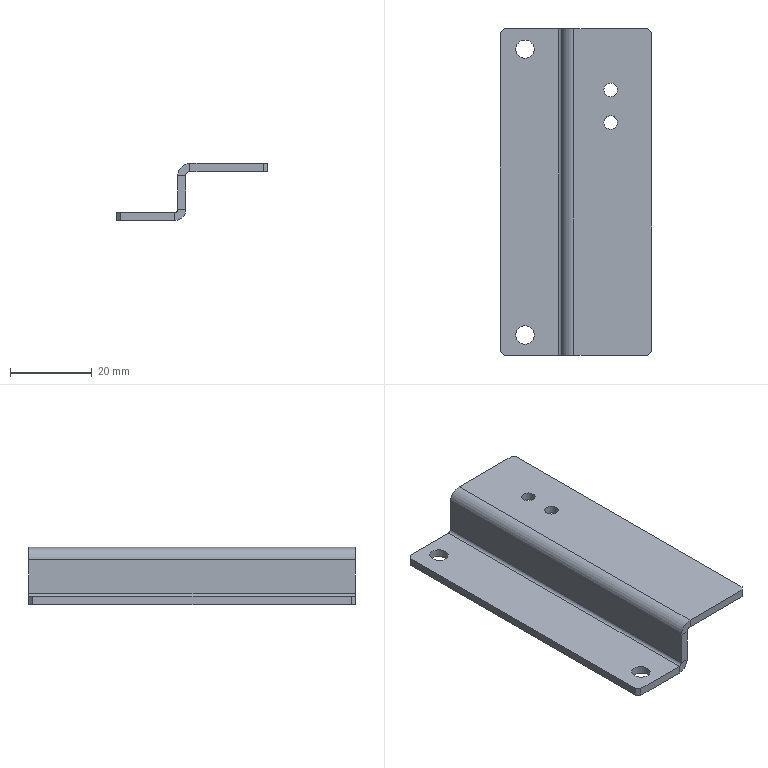Part | NX | 1 solid | 30 faces | box 37 x 80 x 14 mm | volume 7482 mm3 | plane 22 | cylinder 8 | commonest cylinder face diameters 3.3 x2 4.5 x2 1.473 x1 2 x1 5.473 x1 6 x1
STEP:
#1=CARTESIAN_POINT('',(-12.,-40.,-3.));
#2=VERTEX_POINT('',#1);
#3=CARTESIAN_POINT('',(-12.,-40.,-11.263));
#4=VERTEX_POINT('',#3);
#5=CARTESIAN_POINT('',(-12.,-40.,-12.));
#6=DIRECTION('',(0.,0.,-1.));
#7=VECTOR('',#6,1000.);
#8=LINE('',#5,#7);
#9=EDGE_CURVE('',#2,#4,#8,.T.);
#10=ORIENTED_EDGE('',*,*,#9,.T.);
#11=CARTESIAN_POINT('',(-10.,-40.,-11.263));
#12=VERTEX_POINT('',#11);
#13=CARTESIAN_POINT('',(-12.,-40.,-11.263));
#14=DIRECTION('',(1.,0.,0.));
#15=VECTOR('',#14,1000.);
#16=LINE('',#13,#15);
#17=EDGE_CURVE('',#4,#12,#16,.T.);
#18=ORIENTED_EDGE('',*,*,#17,.T.);
#19=CARTESIAN_POINT('',(-10.,-40.,-3.));
#20=VERTEX_POINT('',#19);
#21=CARTESIAN_POINT('',(-10.,-40.,-12.));
#22=DIRECTION('',(0.,0.,-1.));
#23=VECTOR('',#22,1000.);
#24=LINE('',#21,#23);
#25=EDGE_CURVE('',#20,#12,#24,.T.);
#26=ORIENTED_EDGE('',*,*,#25,.F.);
#27=CARTESIAN_POINT('',(-10.,-40.,-3.));
#28=DIRECTION('',(-1.,0.,0.));
#29=VECTOR('',#28,1000.);
#30=LINE('',#27,#29);
#31=EDGE_CURVE('',#20,#2,#30,.T.);
#32=ORIENTED_EDGE('',*,*,#31,.T.);
#33=EDGE_LOOP('',(#10,#18,#26,#32));
#34=FACE_BOUND('',#33,.T.);
#35=CARTESIAN_POINT('',(-12.,-40.,-12.));
#36=DIRECTION('',(0.,-1.,0.));
#37=DIRECTION('',(0.,0.,-1.));
#38=AXIS2_PLACEMENT_3D('',#35,#36,#37);
#39=PLANE('',#38);
#40=ADVANCED_FACE('',(#34),#39,.T.);
#41=CARTESIAN_POINT('',(-12.,40.,-11.263));
#42=VERTEX_POINT('',#41);
#43=CARTESIAN_POINT('',(-12.,40.,-3.));
#44=VERTEX_POINT('',#43);
#45=CARTESIAN_POINT('',(-12.,40.,-2.));
#46=DIRECTION('',(0.,0.,1.));
#47=VECTOR('',#46,1000.);
#48=LINE('',#45,#47);
#49=EDGE_CURVE('',#42,#44,#48,.T.);
#50=ORIENTED_EDGE('',*,*,#49,.F.);
#51=CARTESIAN_POINT('',(-12.,-40.,-11.263));
#52=DIRECTION('',(0.,-1.,0.));
#53=VECTOR('',#52,1000.);
#54=LINE('',#51,#53);
#55=EDGE_CURVE('',#4,#42,#54,.F.);
#56=ORIENTED_EDGE('',*,*,#55,.F.);
#57=ORIENTED_EDGE('',*,*,#9,.F.);
#58=CARTESIAN_POINT('',(-12.,0.,-3.));
#59=DIRECTION('',(0.,1.,0.));
#60=VECTOR('',#59,1000.);
#61=LINE('',#58,#60);
#62=EDGE_CURVE('',#2,#44,#61,.T.);
#63=ORIENTED_EDGE('',*,*,#62,.T.);
#64=EDGE_LOOP('',(#50,#56,#57,#63));
#65=FACE_BOUND('',#64,.T.);
#66=CARTESIAN_POINT('',(-12.,0.,0.));
#67=DIRECTION('',(-1.,0.,0.));
#68=DIRECTION('',(0.,0.,1.));
#69=AXIS2_PLACEMENT_3D('',#66,#67,#68);
#70=PLANE('',#69);
#71=ADVANCED_FACE('',(#65),#70,.T.);
#72=CARTESIAN_POINT('',(-10.,40.,-11.263));
#73=VERTEX_POINT('',#72);
#74=CARTESIAN_POINT('',(-10.,-40.,-11.263));
#75=DIRECTION('',(0.,-1.,0.));
#76=VECTOR('',#75,1000.);
#77=LINE('',#74,#76);
#78=EDGE_CURVE('',#12,#73,#77,.F.);
#79=ORIENTED_EDGE('',*,*,#78,.T.);
#80=CARTESIAN_POINT('',(-10.,40.,-3.));
#81=VERTEX_POINT('',#80);
#82=CARTESIAN_POINT('',(-10.,40.,-2.));
#83=DIRECTION('',(0.,0.,1.));
#84=VECTOR('',#83,1000.);
#85=LINE('',#82,#84);
#86=EDGE_CURVE('',#73,#81,#85,.T.);
#87=ORIENTED_EDGE('',*,*,#86,.T.);
#88=CARTESIAN_POINT('',(-10.,-40.,-3.));
#89=DIRECTION('',(0.,1.,0.));
#90=VECTOR('',#89,1000.);
#91=LINE('',#88,#90);
#92=EDGE_CURVE('',#20,#81,#91,.T.);
#93=ORIENTED_EDGE('',*,*,#92,.F.);
#94=ORIENTED_EDGE('',*,*,#25,.T.);
#95=EDGE_LOOP('',(#79,#87,#93,#94));
#96=FACE_BOUND('',#95,.T.);
#97=CARTESIAN_POINT('',(-10.,0.,0.));
#98=DIRECTION('',(-1.,0.,0.));
#99=DIRECTION('',(0.,0.,1.));
#100=AXIS2_PLACEMENT_3D('',#97,#98,#99);
#101=PLANE('',#100);
#102=ADVANCED_FACE('',(#96),#101,.F.);
#103=CARTESIAN_POINT('',(9.,40.,0.));
#104=VERTEX_POINT('',#103);
#105=CARTESIAN_POINT('',(-9.,40.,0.));
#106=VERTEX_POINT('',#105);
#107=CARTESIAN_POINT('',(-10.,40.,0.));
#108=DIRECTION('',(-1.,0.,0.));
#109=VECTOR('',#108,1000.);
#110=LINE('',#107,#109);
#111=EDGE_CURVE('',#104,#106,#110,.T.);
#112=ORIENTED_EDGE('',*,*,#111,.F.);
#113=CARTESIAN_POINT('',(9.,40.,-2.));
#114=VERTEX_POINT('',#113);
#115=CARTESIAN_POINT('',(9.,40.,-2.));
#116=DIRECTION('',(0.,0.,-1.));
#117=VECTOR('',#116,1000.);
#118=LINE('',#115,#117);
#119=EDGE_CURVE('',#104,#114,#118,.T.);
#120=ORIENTED_EDGE('',*,*,#119,.T.);
#121=CARTESIAN_POINT('',(-9.,40.,-2.));
#122=VERTEX_POINT('',#121);
#123=CARTESIAN_POINT('',(-10.,40.,-2.));
#124=DIRECTION('',(-1.,0.,0.));
#125=VECTOR('',#124,1000.);
#126=LINE('',#123,#125);
#127=EDGE_CURVE('',#114,#122,#126,.T.);
#128=ORIENTED_EDGE('',*,*,#127,.T.);
#129=CARTESIAN_POINT('',(-9.,40.,-2.));
#130=DIRECTION('',(0.,0.,1.));
#131=VECTOR('',#130,1000.);
#132=LINE('',#129,#131);
#133=EDGE_CURVE('',#122,#106,#132,.T.);
#134=ORIENTED_EDGE('',*,*,#133,.T.);
#135=EDGE_LOOP('',(#112,#120,#128,#134));
#136=FACE_BOUND('',#135,.T.);
#137=CARTESIAN_POINT('',(-10.,40.,-2.));
#138=DIRECTION('',(0.,1.,0.));
#139=DIRECTION('',(0.,0.,1.));
#140=AXIS2_PLACEMENT_3D('',#137,#138,#139);
#141=PLANE('',#140);
#142=ADVANCED_FACE('',(#136),#141,.T.);
#143=CARTESIAN_POINT('',(1.65,17.,-2.));
#144=VERTEX_POINT('',#143);
#145=CARTESIAN_POINT('',(0.,17.,-2.));
#146=DIRECTION('',(0.,0.,1.));
#147=DIRECTION('',(1.,0.,0.));
#148=AXIS2_PLACEMENT_3D('',#145,#146,#147);
#149=CIRCLE('',#148,1.65);
#150=EDGE_CURVE('',#144,#144,#149,.T.);
#151=ORIENTED_EDGE('',*,*,#150,.T.);
#152=EDGE_LOOP('',(#151));
#153=FACE_BOUND('',#152,.T.);
#154=CARTESIAN_POINT('',(1.65,25.,-2.));
#155=VERTEX_POINT('',#154);
#156=CARTESIAN_POINT('',(0.,25.,-2.));
#157=DIRECTION('',(0.,0.,1.));
#158=DIRECTION('',(1.,0.,0.));
#159=AXIS2_PLACEMENT_3D('',#156,#157,#158);
#160=CIRCLE('',#159,1.65);
#161=EDGE_CURVE('',#155,#155,#160,.T.);
#162=ORIENTED_EDGE('',*,*,#161,.T.);
#163=EDGE_LOOP('',(#162));
#164=FACE_BOUND('',#163,.T.);
#165=CARTESIAN_POINT('',(10.,-39.,-2.));
#166=VERTEX_POINT('',#165);
#167=CARTESIAN_POINT('',(10.,39.,-2.));
#168=VERTEX_POINT('',#167);
#169=CARTESIAN_POINT('',(10.,-40.,-2.));
#170=DIRECTION('',(0.,1.,0.));
#171=VECTOR('',#170,1000.);
#172=LINE('',#169,#171);
#173=EDGE_CURVE('',#166,#168,#172,.T.);
#174=ORIENTED_EDGE('',*,*,#173,.F.);
#175=CARTESIAN_POINT('',(9.,-40.,-2.));
#176=VERTEX_POINT('',#175);
#177=CARTESIAN_POINT('',(24.5,-24.5,-2.));
#178=DIRECTION('',(0.7071,0.7071,0.));
#179=VECTOR('',#178,1000.);
#180=LINE('',#177,#179);
#181=EDGE_CURVE('',#166,#176,#180,.F.);
#182=ORIENTED_EDGE('',*,*,#181,.T.);
#183=CARTESIAN_POINT('',(-9.,-40.,-2.));
#184=VERTEX_POINT('',#183);
#185=CARTESIAN_POINT('',(-10.,-40.,-2.));
#186=DIRECTION('',(1.,0.,0.));
#187=VECTOR('',#186,1000.);
#188=LINE('',#185,#187);
#189=EDGE_CURVE('',#184,#176,#188,.T.);
#190=ORIENTED_EDGE('',*,*,#189,.F.);
#191=CARTESIAN_POINT('',(-9.,40.,-2.));
#192=DIRECTION('',(0.,1.,0.));
#193=VECTOR('',#192,1000.);
#194=LINE('',#191,#193);
#195=EDGE_CURVE('',#122,#184,#194,.F.);
#196=ORIENTED_EDGE('',*,*,#195,.F.);
#197=ORIENTED_EDGE('',*,*,#127,.F.);
#198=CARTESIAN_POINT('',(24.5,24.5,-2.));
#199=DIRECTION('',(-0.7071,0.7071,0.));
#200=VECTOR('',#199,1000.);
#201=LINE('',#198,#200);
#202=EDGE_CURVE('',#114,#168,#201,.F.);
#203=ORIENTED_EDGE('',*,*,#202,.T.);
#204=EDGE_LOOP('',(#174,#182,#190,#196,#197,#203));
#205=FACE_BOUND('',#204,.T.);
#206=CARTESIAN_POINT('',(0.,0.,-2.));
#207=DIRECTION('',(0.,0.,-1.));
#208=DIRECTION('',(-1.,0.,0.));
#209=AXIS2_PLACEMENT_3D('',#206,#207,#208);
#210=PLANE('',#209);
#211=ADVANCED_FACE('',(#153,#164,#205),#210,.T.);
#212=CARTESIAN_POINT('',(1.65,17.,0.));
#213=VERTEX_POINT('',#212);
#214=CARTESIAN_POINT('',(0.,17.,0.));
#215=DIRECTION('',(0.,0.,1.));
#216=DIRECTION('',(1.,0.,0.));
#217=AXIS2_PLACEMENT_3D('',#214,#215,#216);
#218=CIRCLE('',#217,1.65);
#219=EDGE_CURVE('',#213,#213,#218,.T.);
#220=ORIENTED_EDGE('',*,*,#219,.F.);
#221=EDGE_LOOP('',(#220));
#222=FACE_BOUND('',#221,.T.);
#223=CARTESIAN_POINT('',(1.65,25.,0.));
#224=VERTEX_POINT('',#223);
#225=CARTESIAN_POINT('',(0.,25.,0.));
#226=DIRECTION('',(0.,0.,1.));
#227=DIRECTION('',(1.,0.,0.));
#228=AXIS2_PLACEMENT_3D('',#225,#226,#227);
#229=CIRCLE('',#228,1.65);
#230=EDGE_CURVE('',#224,#224,#229,.T.);
#231=ORIENTED_EDGE('',*,*,#230,.F.);
#232=EDGE_LOOP('',(#231));
#233=FACE_BOUND('',#232,.T.);
#234=CARTESIAN_POINT('',(-9.,-40.,0.));
#235=VERTEX_POINT('',#234);
#236=CARTESIAN_POINT('',(9.,-40.,0.));
#237=VERTEX_POINT('',#236);
#238=CARTESIAN_POINT('',(-10.,-40.,0.));
#239=DIRECTION('',(1.,0.,0.));
#240=VECTOR('',#239,1000.);
#241=LINE('',#238,#240);
#242=EDGE_CURVE('',#235,#237,#241,.T.);
#243=ORIENTED_EDGE('',*,*,#242,.T.);
#244=CARTESIAN_POINT('',(10.,-39.,0.));
#245=VERTEX_POINT('',#244);
#246=CARTESIAN_POINT('',(9.,-40.,0.));
#247=DIRECTION('',(-0.7071,-0.7071,0.));
#248=VECTOR('',#247,1000.);
#249=LINE('',#246,#248);
#250=EDGE_CURVE('',#237,#245,#249,.F.);
#251=ORIENTED_EDGE('',*,*,#250,.T.);
#252=CARTESIAN_POINT('',(10.,39.,0.));
#253=VERTEX_POINT('',#252);
#254=CARTESIAN_POINT('',(10.,-40.,0.));
#255=DIRECTION('',(0.,1.,0.));
#256=VECTOR('',#255,1000.);
#257=LINE('',#254,#256);
#258=EDGE_CURVE('',#245,#253,#257,.T.);
#259=ORIENTED_EDGE('',*,*,#258,.T.);
#260=CARTESIAN_POINT('',(10.,39.,0.));
#261=DIRECTION('',(0.7071,-0.7071,0.));
#262=VECTOR('',#261,1000.);
#263=LINE('',#260,#262);
#264=EDGE_CURVE('',#253,#104,#263,.F.);
#265=ORIENTED_EDGE('',*,*,#264,.T.);
#266=ORIENTED_EDGE('',*,*,#111,.T.);
#267=CARTESIAN_POINT('',(-9.,40.,0.));
#268=DIRECTION('',(0.,1.,0.));
#269=VECTOR('',#268,1000.);
#270=LINE('',#267,#269);
#271=EDGE_CURVE('',#106,#235,#270,.F.);
#272=ORIENTED_EDGE('',*,*,#271,.T.);
#273=EDGE_LOOP('',(#243,#251,#259,#265,#266,#272));
#274=FACE_BOUND('',#273,.T.);
#275=CARTESIAN_POINT('',(0.,0.,0.));
#276=DIRECTION('',(0.,0.,-1.));
#277=DIRECTION('',(-1.,0.,0.));
#278=AXIS2_PLACEMENT_3D('',#275,#276,#277);
#279=PLANE('',#278);
#280=ADVANCED_FACE('',(#222,#233,#274),#279,.F.);
#281=ORIENTED_EDGE('',*,*,#258,.F.);
#282=CARTESIAN_POINT('',(10.,-39.,-2.));
#283=DIRECTION('',(0.,0.,-1.));
#284=VECTOR('',#283,1000.);
#285=LINE('',#282,#284);
#286=EDGE_CURVE('',#245,#166,#285,.T.);
#287=ORIENTED_EDGE('',*,*,#286,.T.);
#288=ORIENTED_EDGE('',*,*,#173,.T.);
#289=CARTESIAN_POINT('',(10.,39.,-2.));
#290=DIRECTION('',(0.,0.,1.));
#291=VECTOR('',#290,1000.);
#292=LINE('',#289,#291);
#293=EDGE_CURVE('',#168,#253,#292,.T.);
#294=ORIENTED_EDGE('',*,*,#293,.T.);
#295=EDGE_LOOP('',(#281,#287,#288,#294));
#296=FACE_BOUND('',#295,.T.);
#297=CARTESIAN_POINT('',(10.,-40.,-2.));
#298=DIRECTION('',(1.,0.,0.));
#299=DIRECTION('',(0.,0.,-1.));
#300=AXIS2_PLACEMENT_3D('',#297,#298,#299);
#301=PLANE('',#300);
#302=ADVANCED_FACE('',(#296),#301,.T.);
#303=ORIENTED_EDGE('',*,*,#189,.T.);
#304=CARTESIAN_POINT('',(9.,-40.,-2.));
#305=DIRECTION('',(0.,0.,1.));
#306=VECTOR('',#305,1000.);
#307=LINE('',#304,#306);
#308=EDGE_CURVE('',#176,#237,#307,.T.);
#309=ORIENTED_EDGE('',*,*,#308,.T.);
#310=ORIENTED_EDGE('',*,*,#242,.F.);
#311=CARTESIAN_POINT('',(-9.,-40.,-2.));
#312=DIRECTION('',(0.,0.,1.));
#313=VECTOR('',#312,1000.);
#314=LINE('',#311,#313);
#315=EDGE_CURVE('',#184,#235,#314,.T.);
#316=ORIENTED_EDGE('',*,*,#315,.F.);
#317=EDGE_LOOP('',(#303,#309,#310,#316));
#318=FACE_BOUND('',#317,.T.);
#319=CARTESIAN_POINT('',(-10.,-40.,-2.));
#320=DIRECTION('',(0.,-1.,0.));
#321=DIRECTION('',(0.,0.,-1.));
#322=AXIS2_PLACEMENT_3D('',#319,#320,#321);
#323=PLANE('',#322);
#324=ADVANCED_FACE('',(#318),#323,.T.);
#325=ORIENTED_EDGE('',*,*,#150,.F.);
#326=EDGE_LOOP('',(#325));
#327=FACE_BOUND('',#326,.T.);
#328=ORIENTED_EDGE('',*,*,#219,.T.);
#329=EDGE_LOOP('',(#328));
#330=FACE_BOUND('',#329,.T.);
#331=CARTESIAN_POINT('',(0.,17.,0.));
#332=DIRECTION('',(0.,0.,1.));
#333=DIRECTION('',(1.,0.,0.));
#334=AXIS2_PLACEMENT_3D('',#331,#332,#333);
#335=CYLINDRICAL_SURFACE('',#334,1.65);
#336=ADVANCED_FACE('',(#327,#330),#335,.F.);
#337=ORIENTED_EDGE('',*,*,#161,.F.);
#338=EDGE_LOOP('',(#337));
#339=FACE_BOUND('',#338,.T.);
#340=ORIENTED_EDGE('',*,*,#230,.T.);
#341=EDGE_LOOP('',(#340));
#342=FACE_BOUND('',#341,.T.);
#343=CARTESIAN_POINT('',(0.,25.,0.));
#344=DIRECTION('',(0.,0.,1.));
#345=DIRECTION('',(1.,0.,0.));
#346=AXIS2_PLACEMENT_3D('',#343,#344,#345);
#347=CYLINDRICAL_SURFACE('',#346,1.65);
#348=ADVANCED_FACE('',(#339,#342),#347,.F.);
#349=ORIENTED_EDGE('',*,*,#31,.F.);
#350=CARTESIAN_POINT('',(-9.,-40.,-3.));
#351=DIRECTION('',(0.,1.,0.));
#352=DIRECTION('',(0.,0.,1.));
#353=AXIS2_PLACEMENT_3D('',#350,#351,#352);
#354=CIRCLE('',#353,1.);
#355=EDGE_CURVE('',#184,#20,#354,.F.);
#356=ORIENTED_EDGE('',*,*,#355,.F.);
#357=ORIENTED_EDGE('',*,*,#315,.T.);
#358=CARTESIAN_POINT('',(-9.,-40.,-3.));
#359=DIRECTION('',(0.,1.,0.));
#360=DIRECTION('',(0.,0.,1.));
#361=AXIS2_PLACEMENT_3D('',#358,#359,#360);
#362=CIRCLE('',#361,3.);
#363=EDGE_CURVE('',#235,#2,#362,.F.);
#364=ORIENTED_EDGE('',*,*,#363,.T.);
#365=EDGE_LOOP('',(#349,#356,#357,#364));
#366=FACE_BOUND('',#365,.T.);
#367=CARTESIAN_POINT('',(-9.,-40.,-3.));
#368=DIRECTION('',(0.,-1.,0.));
#369=DIRECTION('',(0.,0.,-1.));
#370=AXIS2_PLACEMENT_3D('',#367,#368,#369);
#371=PLANE('',#370);
#372=ADVANCED_FACE('',(#366),#371,.T.);
#373=CARTESIAN_POINT('',(-9.,40.,-3.));
#374=DIRECTION('',(0.,1.,0.));
#375=DIRECTION('',(0.,0.,1.));
#376=AXIS2_PLACEMENT_3D('',#373,#374,#375);
#377=CIRCLE('',#376,1.);
#378=EDGE_CURVE('',#81,#122,#377,.T.);
#379=ORIENTED_EDGE('',*,*,#378,.F.);
#380=CARTESIAN_POINT('',(-10.,40.,-3.));
#381=DIRECTION('',(-1.,0.,0.));
#382=VECTOR('',#381,1000.);
#383=LINE('',#380,#382);
#384=EDGE_CURVE('',#81,#44,#383,.T.);
#385=ORIENTED_EDGE('',*,*,#384,.T.);
#386=CARTESIAN_POINT('',(-9.,40.,-3.));
#387=DIRECTION('',(0.,1.,0.));
#388=DIRECTION('',(0.,0.,1.));
#389=AXIS2_PLACEMENT_3D('',#386,#387,#388);
#390=CIRCLE('',#389,3.);
#391=EDGE_CURVE('',#44,#106,#390,.T.);
#392=ORIENTED_EDGE('',*,*,#391,.T.);
#393=ORIENTED_EDGE('',*,*,#133,.F.);
#394=EDGE_LOOP('',(#379,#385,#392,#393));
#395=FACE_BOUND('',#394,.T.);
#396=CARTESIAN_POINT('',(-9.,40.,-3.));
#397=DIRECTION('',(0.,-1.,0.));
#398=DIRECTION('',(0.,0.,-1.));
#399=AXIS2_PLACEMENT_3D('',#396,#397,#398);
#400=PLANE('',#399);
#401=ADVANCED_FACE('',(#395),#400,.F.);
#402=ORIENTED_EDGE('',*,*,#271,.F.);
#403=ORIENTED_EDGE('',*,*,#391,.F.);
#404=ORIENTED_EDGE('',*,*,#62,.F.);
#405=ORIENTED_EDGE('',*,*,#363,.F.);
#406=EDGE_LOOP('',(#402,#403,#404,#405));
#407=FACE_BOUND('',#406,.T.);
#408=CARTESIAN_POINT('',(-9.,40.,-3.));
#409=DIRECTION('',(0.,1.,0.));
#410=DIRECTION('',(-1.,0.,0.));
#411=AXIS2_PLACEMENT_3D('',#408,#409,#410);
#412=CYLINDRICAL_SURFACE('',#411,3.);
#413=ADVANCED_FACE('',(#407),#412,.T.);
#414=ORIENTED_EDGE('',*,*,#195,.T.);
#415=ORIENTED_EDGE('',*,*,#355,.T.);
#416=ORIENTED_EDGE('',*,*,#92,.T.);
#417=ORIENTED_EDGE('',*,*,#378,.T.);
#418=EDGE_LOOP('',(#414,#415,#416,#417));
#419=FACE_BOUND('',#418,.T.);
#420=CARTESIAN_POINT('',(-9.,40.,-3.));
#421=DIRECTION('',(0.,1.,0.));
#422=DIRECTION('',(-1.,0.,0.));
#423=AXIS2_PLACEMENT_3D('',#420,#421,#422);
#424=CYLINDRICAL_SURFACE('',#423,1.);
#425=ADVANCED_FACE('',(#419),#424,.F.);
#426=CARTESIAN_POINT('',(-12.,40.,-11.263));
#427=DIRECTION('',(1.,0.,0.));
#428=VECTOR('',#427,1000.);
#429=LINE('',#426,#428);
#430=EDGE_CURVE('',#42,#73,#429,.T.);
#431=ORIENTED_EDGE('',*,*,#430,.F.);
#432=ORIENTED_EDGE('',*,*,#49,.T.);
#433=ORIENTED_EDGE('',*,*,#384,.F.);
#434=ORIENTED_EDGE('',*,*,#86,.F.);
#435=EDGE_LOOP('',(#431,#432,#433,#434));
#436=FACE_BOUND('',#435,.T.);
#437=CARTESIAN_POINT('',(-12.,40.,-2.));
#438=DIRECTION('',(0.,1.,0.));
#439=DIRECTION('',(0.,0.,1.));
#440=AXIS2_PLACEMENT_3D('',#437,#438,#439);
#441=PLANE('',#440);
#442=ADVANCED_FACE('',(#436),#441,.T.);
#443=CARTESIAN_POINT('',(-12.737,40.,-12.));
#444=VERTEX_POINT('',#443);
#445=CARTESIAN_POINT('',(-12.737,40.,-14.));
#446=VERTEX_POINT('',#445);
#447=CARTESIAN_POINT('',(-12.737,40.,-12.));
#448=DIRECTION('',(0.,0.,-1.));
#449=VECTOR('',#448,1000.);
#450=LINE('',#447,#449);
#451=EDGE_CURVE('',#444,#446,#450,.T.);
#452=ORIENTED_EDGE('',*,*,#451,.F.);
#453=CARTESIAN_POINT('',(-12.737,40.,-11.263));
#454=DIRECTION('',(0.,-1.,0.));
#455=DIRECTION('',(0.,0.,-1.));
#456=AXIS2_PLACEMENT_3D('',#453,#454,#455);
#457=CIRCLE('',#456,0.7366);
#458=EDGE_CURVE('',#42,#444,#457,.F.);
#459=ORIENTED_EDGE('',*,*,#458,.F.);
#460=ORIENTED_EDGE('',*,*,#430,.T.);
#461=CARTESIAN_POINT('',(-12.737,40.,-11.263));
#462=DIRECTION('',(0.,-1.,0.));
#463=DIRECTION('',(0.,0.,-1.));
#464=AXIS2_PLACEMENT_3D('',#461,#462,#463);
#465=CIRCLE('',#464,2.737);
#466=EDGE_CURVE('',#73,#446,#465,.F.);
#467=ORIENTED_EDGE('',*,*,#466,.T.);
#468=EDGE_LOOP('',(#452,#459,#460,#467));
#469=FACE_BOUND('',#468,.T.);
#470=CARTESIAN_POINT('',(-12.737,40.,-11.263));
#471=DIRECTION('',(0.,1.,0.));
#472=DIRECTION('',(0.,0.,1.));
#473=AXIS2_PLACEMENT_3D('',#470,#471,#472);
#474=PLANE('',#473);
#475=ADVANCED_FACE('',(#469),#474,.T.);
#476=CARTESIAN_POINT('',(-12.737,-40.,-12.));
#477=VERTEX_POINT('',#476);
#478=CARTESIAN_POINT('',(-12.737,-40.,-11.263));
#479=DIRECTION('',(0.,-1.,0.));
#480=DIRECTION('',(0.,0.,-1.));
#481=AXIS2_PLACEMENT_3D('',#478,#479,#480);
#482=CIRCLE('',#481,0.7366);
#483=EDGE_CURVE('',#477,#4,#482,.T.);
#484=ORIENTED_EDGE('',*,*,#483,.F.);
#485=CARTESIAN_POINT('',(-12.737,-40.,-14.));
#486=VERTEX_POINT('',#485);
#487=CARTESIAN_POINT('',(-12.737,-40.,-12.));
#488=DIRECTION('',(0.,0.,-1.));
#489=VECTOR('',#488,1000.);
#490=LINE('',#487,#489);
#491=EDGE_CURVE('',#477,#486,#490,.T.);
#492=ORIENTED_EDGE('',*,*,#491,.T.);
#493=CARTESIAN_POINT('',(-12.737,-40.,-11.263));
#494=DIRECTION('',(0.,-1.,0.));
#495=DIRECTION('',(0.,0.,-1.));
#496=AXIS2_PLACEMENT_3D('',#493,#494,#495);
#497=CIRCLE('',#496,2.737);
#498=EDGE_CURVE('',#486,#12,#497,.T.);
#499=ORIENTED_EDGE('',*,*,#498,.T.);
#500=ORIENTED_EDGE('',*,*,#17,.F.);
#501=EDGE_LOOP('',(#484,#492,#499,#500));
#502=FACE_BOUND('',#501,.T.);
#503=CARTESIAN_POINT('',(-12.737,-40.,-11.263));
#504=DIRECTION('',(0.,1.,0.));
#505=DIRECTION('',(0.,0.,1.));
#506=AXIS2_PLACEMENT_3D('',#503,#504,#505);
#507=PLANE('',#506);
#508=ADVANCED_FACE('',(#502),#507,.F.);
#509=ORIENTED_EDGE('',*,*,#78,.F.);
#510=ORIENTED_EDGE('',*,*,#498,.F.);
#511=CARTESIAN_POINT('',(-12.737,0.,-14.));
#512=DIRECTION('',(0.,-1.,0.));
#513=VECTOR('',#512,1000.);
#514=LINE('',#511,#513);
#515=EDGE_CURVE('',#446,#486,#514,.T.);
#516=ORIENTED_EDGE('',*,*,#515,.F.);
#517=ORIENTED_EDGE('',*,*,#466,.F.);
#518=EDGE_LOOP('',(#509,#510,#516,#517));
#519=FACE_BOUND('',#518,.T.);
#520=CARTESIAN_POINT('',(-12.737,-40.,-11.263));
#521=DIRECTION('',(0.,-1.,0.));
#522=DIRECTION('',(0.,0.,-1.));
#523=AXIS2_PLACEMENT_3D('',#520,#521,#522);
#524=CYLINDRICAL_SURFACE('',#523,2.737);
#525=ADVANCED_FACE('',(#519),#524,.T.);
#526=ORIENTED_EDGE('',*,*,#55,.T.);
#527=ORIENTED_EDGE('',*,*,#458,.T.);
#528=CARTESIAN_POINT('',(-12.737,40.,-12.));
#529=DIRECTION('',(0.,-1.,0.));
#530=VECTOR('',#529,1000.);
#531=LINE('',#528,#530);
#532=EDGE_CURVE('',#444,#477,#531,.T.);
#533=ORIENTED_EDGE('',*,*,#532,.T.);
#534=ORIENTED_EDGE('',*,*,#483,.T.);
#535=EDGE_LOOP('',(#526,#527,#533,#534));
#536=FACE_BOUND('',#535,.T.);
#537=CARTESIAN_POINT('',(-12.737,-40.,-11.263));
#538=DIRECTION('',(0.,-1.,0.));
#539=DIRECTION('',(0.,0.,-1.));
#540=AXIS2_PLACEMENT_3D('',#537,#538,#539);
#541=CYLINDRICAL_SURFACE('',#540,0.7366);
#542=ADVANCED_FACE('',(#536),#541,.F.);
#543=CARTESIAN_POINT('',(-26.,-40.,-12.));
#544=VERTEX_POINT('',#543);
#545=CARTESIAN_POINT('',(-12.,-40.,-12.));
#546=DIRECTION('',(1.,0.,0.));
#547=VECTOR('',#546,1000.);
#548=LINE('',#545,#547);
#549=EDGE_CURVE('',#544,#477,#548,.T.);
#550=ORIENTED_EDGE('',*,*,#549,.F.);
#551=CARTESIAN_POINT('',(-26.,-40.,-14.));
#552=VERTEX_POINT('',#551);
#553=CARTESIAN_POINT('',(-26.,-40.,-14.));
#554=DIRECTION('',(0.,0.,-1.));
#555=VECTOR('',#554,1000.);
#556=LINE('',#553,#555);
#557=EDGE_CURVE('',#544,#552,#556,.T.);
#558=ORIENTED_EDGE('',*,*,#557,.T.);
#559=CARTESIAN_POINT('',(-12.,-40.,-14.));
#560=DIRECTION('',(1.,0.,0.));
#561=VECTOR('',#560,1000.);
#562=LINE('',#559,#561);
#563=EDGE_CURVE('',#552,#486,#562,.T.);
#564=ORIENTED_EDGE('',*,*,#563,.T.);
#565=ORIENTED_EDGE('',*,*,#491,.F.);
#566=EDGE_LOOP('',(#550,#558,#564,#565));
#567=FACE_BOUND('',#566,.T.);
#568=CARTESIAN_POINT('',(-12.,-40.,-14.));
#569=DIRECTION('',(0.,-1.,0.));
#570=DIRECTION('',(0.,0.,-1.));
#571=AXIS2_PLACEMENT_3D('',#568,#569,#570);
#572=PLANE('',#571);
#573=ADVANCED_FACE('',(#567),#572,.T.);
#574=CARTESIAN_POINT('',(-26.,40.,-14.));
#575=VERTEX_POINT('',#574);
#576=CARTESIAN_POINT('',(-27.,40.,-14.));
#577=DIRECTION('',(-1.,0.,0.));
#578=VECTOR('',#577,1000.);
#579=LINE('',#576,#578);
#580=EDGE_CURVE('',#446,#575,#579,.T.);
#581=ORIENTED_EDGE('',*,*,#580,.T.);
#582=CARTESIAN_POINT('',(-26.,40.,-12.));
#583=VERTEX_POINT('',#582);
#584=CARTESIAN_POINT('',(-26.,40.,-14.));
#585=DIRECTION('',(0.,0.,1.));
#586=VECTOR('',#585,1000.);
#587=LINE('',#584,#586);
#588=EDGE_CURVE('',#575,#583,#587,.T.);
#589=ORIENTED_EDGE('',*,*,#588,.T.);
#590=CARTESIAN_POINT('',(-27.,40.,-12.));
#591=DIRECTION('',(-1.,0.,0.));
#592=VECTOR('',#591,1000.);
#593=LINE('',#590,#592);
#594=EDGE_CURVE('',#444,#583,#593,.T.);
#595=ORIENTED_EDGE('',*,*,#594,.F.);
#596=ORIENTED_EDGE('',*,*,#451,.T.);
#597=EDGE_LOOP('',(#581,#589,#595,#596));
#598=FACE_BOUND('',#597,.T.);
#599=CARTESIAN_POINT('',(-27.,40.,-14.));
#600=DIRECTION('',(0.,1.,0.));
#601=DIRECTION('',(-1.,0.,0.));
#602=AXIS2_PLACEMENT_3D('',#599,#600,#601);
#603=PLANE('',#602);
#604=ADVANCED_FACE('',(#598),#603,.T.);
#605=CARTESIAN_POINT('',(-23.25,35.,-14.));
#606=VERTEX_POINT('',#605);
#607=CARTESIAN_POINT('',(-21.,35.,-14.));
#608=DIRECTION('',(0.,0.,-1.));
#609=DIRECTION('',(-1.,0.,0.));
#610=AXIS2_PLACEMENT_3D('',#607,#608,#609);
#611=CIRCLE('',#610,2.25);
#612=EDGE_CURVE('',#606,#606,#611,.T.);
#613=ORIENTED_EDGE('',*,*,#612,.F.);
#614=EDGE_LOOP('',(#613));
#615=FACE_BOUND('',#614,.T.);
#616=CARTESIAN_POINT('',(-23.25,-35.,-14.));
#617=VERTEX_POINT('',#616);
#618=CARTESIAN_POINT('',(-21.,-35.,-14.));
#619=DIRECTION('',(0.,0.,-1.));
#620=DIRECTION('',(-1.,0.,0.));
#621=AXIS2_PLACEMENT_3D('',#618,#619,#620);
#622=CIRCLE('',#621,2.25);
#623=EDGE_CURVE('',#617,#617,#622,.T.);
#624=ORIENTED_EDGE('',*,*,#623,.F.);
#625=EDGE_LOOP('',(#624));
#626=FACE_BOUND('',#625,.T.);
#627=CARTESIAN_POINT('',(-27.,39.,-14.));
#628=VERTEX_POINT('',#627);
#629=CARTESIAN_POINT('',(-27.,-39.,-14.));
#630=VERTEX_POINT('',#629);
#631=CARTESIAN_POINT('',(-27.,-40.,-14.));
#632=DIRECTION('',(0.,-1.,0.));
#633=VECTOR('',#632,1000.);
#634=LINE('',#631,#633);
#635=EDGE_CURVE('',#628,#630,#634,.T.);
#636=ORIENTED_EDGE('',*,*,#635,.F.);
#637=CARTESIAN_POINT('',(-33.,33.,-14.));
#638=DIRECTION('',(-0.7071,-0.7071,0.));
#639=VECTOR('',#638,1000.);
#640=LINE('',#637,#639);
#641=EDGE_CURVE('',#628,#575,#640,.F.);
#642=ORIENTED_EDGE('',*,*,#641,.T.);
#643=ORIENTED_EDGE('',*,*,#580,.F.);
#644=ORIENTED_EDGE('',*,*,#515,.T.);
#645=ORIENTED_EDGE('',*,*,#563,.F.);
#646=CARTESIAN_POINT('',(-33.,-33.,-14.));
#647=DIRECTION('',(0.7071,-0.7071,0.));
#648=VECTOR('',#647,1000.);
#649=LINE('',#646,#648);
#650=EDGE_CURVE('',#552,#630,#649,.F.);
#651=ORIENTED_EDGE('',*,*,#650,.T.);
#652=EDGE_LOOP('',(#636,#642,#643,#644,#645,#651));
#653=FACE_BOUND('',#652,.T.);
#654=CARTESIAN_POINT('',(0.,0.,-14.));
#655=DIRECTION('',(0.,0.,-1.));
#656=DIRECTION('',(-1.,0.,0.));
#657=AXIS2_PLACEMENT_3D('',#654,#655,#656);
#658=PLANE('',#657);
#659=ADVANCED_FACE('',(#615,#626,#653),#658,.T.);
#660=CARTESIAN_POINT('',(-23.25,35.,-12.));
#661=VERTEX_POINT('',#660);
#662=CARTESIAN_POINT('',(-21.,35.,-12.));
#663=DIRECTION('',(0.,0.,-1.));
#664=DIRECTION('',(-1.,0.,0.));
#665=AXIS2_PLACEMENT_3D('',#662,#663,#664);
#666=CIRCLE('',#665,2.25);
#667=EDGE_CURVE('',#661,#661,#666,.T.);
#668=ORIENTED_EDGE('',*,*,#667,.T.);
#669=EDGE_LOOP('',(#668));
#670=FACE_BOUND('',#669,.T.);
#671=CARTESIAN_POINT('',(-23.25,-35.,-12.));
#672=VERTEX_POINT('',#671);
#673=CARTESIAN_POINT('',(-21.,-35.,-12.));
#674=DIRECTION('',(0.,0.,-1.));
#675=DIRECTION('',(-1.,0.,0.));
#676=AXIS2_PLACEMENT_3D('',#673,#674,#675);
#677=CIRCLE('',#676,2.25);
#678=EDGE_CURVE('',#672,#672,#677,.T.);
#679=ORIENTED_EDGE('',*,*,#678,.T.);
#680=EDGE_LOOP('',(#679));
#681=FACE_BOUND('',#680,.T.);
#682=ORIENTED_EDGE('',*,*,#594,.T.);
#683=CARTESIAN_POINT('',(-27.,39.,-12.));
#684=VERTEX_POINT('',#683);
#685=CARTESIAN_POINT('',(-26.,40.,-12.));
#686=DIRECTION('',(0.7071,0.7071,0.));
#687=VECTOR('',#686,1000.);
#688=LINE('',#685,#687);
#689=EDGE_CURVE('',#583,#684,#688,.F.);
#690=ORIENTED_EDGE('',*,*,#689,.T.);
#691=CARTESIAN_POINT('',(-27.,-39.,-12.));
#692=VERTEX_POINT('',#691);
#693=CARTESIAN_POINT('',(-27.,-40.,-12.));
#694=DIRECTION('',(0.,-1.,0.));
#695=VECTOR('',#694,1000.);
#696=LINE('',#693,#695);
#697=EDGE_CURVE('',#684,#692,#696,.T.);
#698=ORIENTED_EDGE('',*,*,#697,.T.);
#699=CARTESIAN_POINT('',(-27.,-39.,-12.));
#700=DIRECTION('',(-0.7071,0.7071,0.));
#701=VECTOR('',#700,1000.);
#702=LINE('',#699,#701);
#703=EDGE_CURVE('',#692,#544,#702,.F.);
#704=ORIENTED_EDGE('',*,*,#703,.T.);
#705=ORIENTED_EDGE('',*,*,#549,.T.);
#706=ORIENTED_EDGE('',*,*,#532,.F.);
#707=EDGE_LOOP('',(#682,#690,#698,#704,#705,#706));
#708=FACE_BOUND('',#707,.T.);
#709=CARTESIAN_POINT('',(0.,0.,-12.));
#710=DIRECTION('',(0.,0.,-1.));
#711=DIRECTION('',(-1.,0.,0.));
#712=AXIS2_PLACEMENT_3D('',#709,#710,#711);
#713=PLANE('',#712);
#714=ADVANCED_FACE('',(#670,#681,#708),#713,.F.);
#715=ORIENTED_EDGE('',*,*,#697,.F.);
#716=CARTESIAN_POINT('',(-27.,39.,-14.));
#717=DIRECTION('',(0.,0.,-1.));
#718=VECTOR('',#717,1000.);
#719=LINE('',#716,#718);
#720=EDGE_CURVE('',#684,#628,#719,.T.);
#721=ORIENTED_EDGE('',*,*,#720,.T.);
#722=ORIENTED_EDGE('',*,*,#635,.T.);
#723=CARTESIAN_POINT('',(-27.,-39.,-14.));
#724=DIRECTION('',(0.,0.,1.));
#725=VECTOR('',#724,1000.);
#726=LINE('',#723,#725);
#727=EDGE_CURVE('',#630,#692,#726,.T.);
#728=ORIENTED_EDGE('',*,*,#727,.T.);
#729=EDGE_LOOP('',(#715,#721,#722,#728));
#730=FACE_BOUND('',#729,.T.);
#731=CARTESIAN_POINT('',(-27.,-40.,-14.));
#732=DIRECTION('',(-1.,0.,0.));
#733=DIRECTION('',(0.,0.,1.));
#734=AXIS2_PLACEMENT_3D('',#731,#732,#733);
#735=PLANE('',#734);
#736=ADVANCED_FACE('',(#730),#735,.T.);
#737=ORIENTED_EDGE('',*,*,#623,.T.);
#738=EDGE_LOOP('',(#737));
#739=FACE_BOUND('',#738,.T.);
#740=ORIENTED_EDGE('',*,*,#678,.F.);
#741=EDGE_LOOP('',(#740));
#742=FACE_BOUND('',#741,.T.);
#743=CARTESIAN_POINT('',(-21.,-35.,-14.));
#744=DIRECTION('',(0.,0.,-1.));
#745=DIRECTION('',(-1.,0.,0.));
#746=AXIS2_PLACEMENT_3D('',#743,#744,#745);
#747=CYLINDRICAL_SURFACE('',#746,2.25);
#748=ADVANCED_FACE('',(#739,#742),#747,.F.);
#749=ORIENTED_EDGE('',*,*,#612,.T.);
#750=EDGE_LOOP('',(#749));
#751=FACE_BOUND('',#750,.T.);
#752=ORIENTED_EDGE('',*,*,#667,.F.);
#753=EDGE_LOOP('',(#752));
#754=FACE_BOUND('',#753,.T.);
#755=CARTESIAN_POINT('',(-21.,35.,-14.));
#756=DIRECTION('',(0.,0.,-1.));
#757=DIRECTION('',(-1.,0.,0.));
#758=AXIS2_PLACEMENT_3D('',#755,#756,#757);
#759=CYLINDRICAL_SURFACE('',#758,2.25);
#760=ADVANCED_FACE('',(#751,#754),#759,.F.);
#761=ORIENTED_EDGE('',*,*,#641,.F.);
#762=ORIENTED_EDGE('',*,*,#720,.F.);
#763=ORIENTED_EDGE('',*,*,#689,.F.);
#764=ORIENTED_EDGE('',*,*,#588,.F.);
#765=EDGE_LOOP('',(#761,#762,#763,#764));
#766=FACE_BOUND('',#765,.T.);
#767=CARTESIAN_POINT('',(-26.,40.,-14.));
#768=DIRECTION('',(0.7071,-0.7071,0.));
#769=DIRECTION('',(0.,0.,1.));
#770=AXIS2_PLACEMENT_3D('',#767,#768,#769);
#771=PLANE('',#770);
#772=ADVANCED_FACE('',(#766),#771,.F.);
#773=ORIENTED_EDGE('',*,*,#650,.F.);
#774=ORIENTED_EDGE('',*,*,#557,.F.);
#775=ORIENTED_EDGE('',*,*,#703,.F.);
#776=ORIENTED_EDGE('',*,*,#727,.F.);
#777=EDGE_LOOP('',(#773,#774,#775,#776));
#778=FACE_BOUND('',#777,.T.);
#779=CARTESIAN_POINT('',(-27.,-39.,-14.));
#780=DIRECTION('',(0.7071,0.7071,0.));
#781=DIRECTION('',(0.,0.,1.));
#782=AXIS2_PLACEMENT_3D('',#779,#780,#781);
#783=PLANE('',#782);
#784=ADVANCED_FACE('',(#778),#783,.F.);
#785=ORIENTED_EDGE('',*,*,#181,.F.);
#786=ORIENTED_EDGE('',*,*,#286,.F.);
#787=ORIENTED_EDGE('',*,*,#250,.F.);
#788=ORIENTED_EDGE('',*,*,#308,.F.);
#789=EDGE_LOOP('',(#785,#786,#787,#788));
#790=FACE_BOUND('',#789,.T.);
#791=CARTESIAN_POINT('',(9.,-40.,-2.));
#792=DIRECTION('',(-0.7071,0.7071,0.));
#793=DIRECTION('',(0.,0.,1.));
#794=AXIS2_PLACEMENT_3D('',#791,#792,#793);
#795=PLANE('',#794);
#796=ADVANCED_FACE('',(#790),#795,.F.);
#797=ORIENTED_EDGE('',*,*,#202,.F.);
#798=ORIENTED_EDGE('',*,*,#119,.F.);
#799=ORIENTED_EDGE('',*,*,#264,.F.);
#800=ORIENTED_EDGE('',*,*,#293,.F.);
#801=EDGE_LOOP('',(#797,#798,#799,#800));
#802=FACE_BOUND('',#801,.T.);
#803=CARTESIAN_POINT('',(10.,39.,-2.));
#804=DIRECTION('',(-0.7071,-0.7071,0.));
#805=DIRECTION('',(0.,0.,1.));
#806=AXIS2_PLACEMENT_3D('',#803,#804,#805);
#807=PLANE('',#806);
#808=ADVANCED_FACE('',(#802),#807,.F.);
#809=CLOSED_SHELL('',(#40,#71,#102,#142,#211,#280,#302,#324,#336,#348,#372,#401,#413,#425,#442,#475,#508,#525,#542,#573,#604,#659,#714,#736,#748,#760,#772,#784,#796,#808));
#810=MANIFOLD_SOLID_BREP('',#809);
#811=(LENGTH_UNIT()NAMED_UNIT(*)SI_UNIT(.MILLI.,.METRE.));
#812=UNCERTAINTY_MEASURE_WITH_UNIT(LENGTH_MEASURE(0.00001),#811,'','');
#813=(NAMED_UNIT(*)PLANE_ANGLE_UNIT()SI_UNIT($,.RADIAN.));
#814=(NAMED_UNIT(*)SI_UNIT($,.STERADIAN.)SOLID_ANGLE_UNIT());
#815=(GEOMETRIC_REPRESENTATION_CONTEXT(3)GLOBAL_UNCERTAINTY_ASSIGNED_CONTEXT((#812))GLOBAL_UNIT_ASSIGNED_CONTEXT((#811,#813,#814))REPRESENTATION_CONTEXT('',''));
#816=ADVANCED_BREP_SHAPE_REPRESENTATION('',(#810),#815);